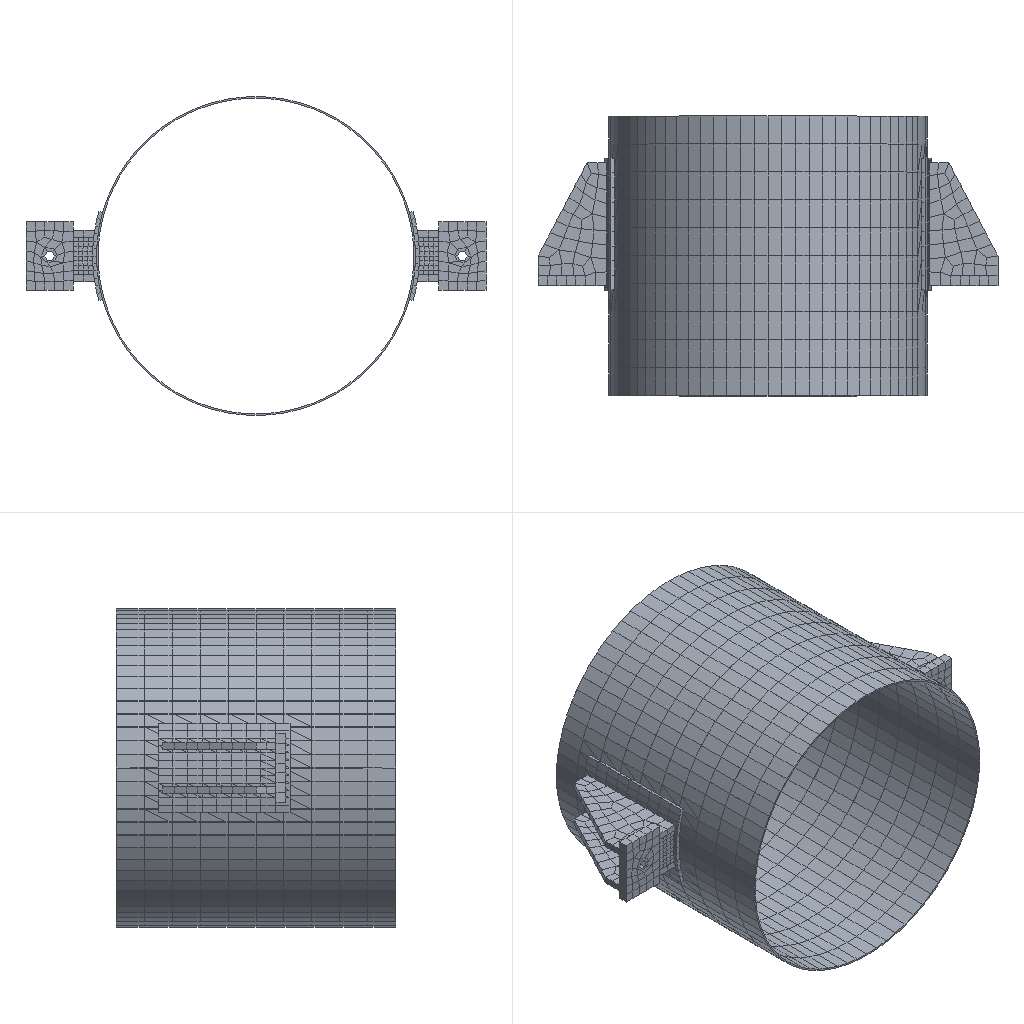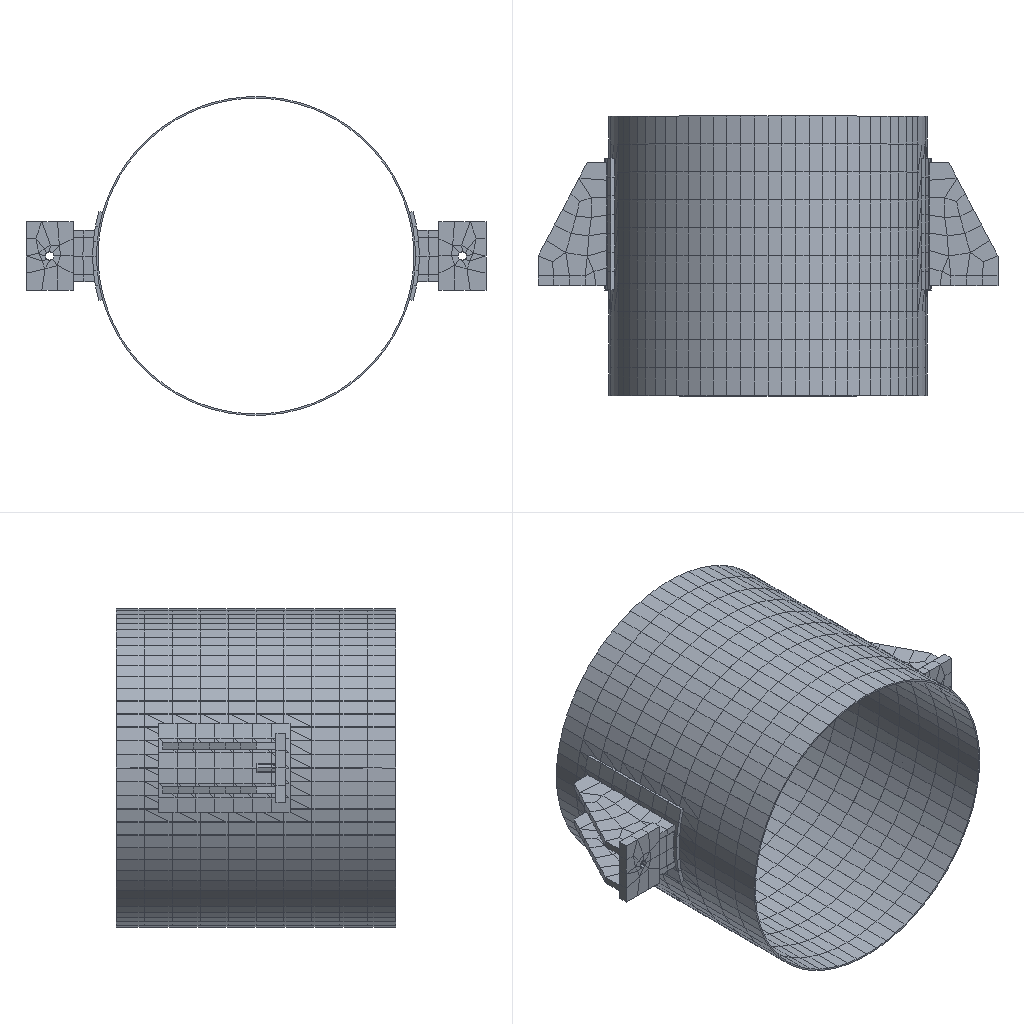Simulation study | ansys workbench
Set-up summary:
category,name,step,type,value,unit,region
solver,ansys_workbench
units,mm-N-s-tonne (MPa),,stated,"/units,MPA"
analysis,deck-1/LS1,,static
load_step,deck-1/LS1,deck-1/LS1,static,nsubst=1; time=1
analysis,deck-2/LS1,,static
load_step,deck-2/LS1,deck-2/LS1,static,nsubst=1; time=1
analysis,deck-3/LS1,,static
load_step,deck-3/LS1,deck-3/LS1,static,nsubst=1; time=1
mesh,deck-1.dat,,nodes,10142
mesh,deck-1.dat,,elements,2684
element_type,SOLID186,,,1302,,deck-1.dat
element_type,TARGE170,,,648,,deck-1.dat
element_type,CONTA174,,,648,,deck-1.dat
element_type,SURF154,,,86,,deck-1.dat
mesh,deck-2.dat,,nodes,10142
mesh,deck-2.dat,,elements,2684
element_type,SOLID186,,,1302,,deck-2.dat
element_type,TARGE170,,,648,,deck-2.dat
element_type,CONTA174,,,648,,deck-2.dat
element_type,SURF154,,,86,,deck-2.dat
mesh,deck-3.dat,,nodes,7696
mesh,deck-3.dat,,elements,1736
element_type,SOLID186,,,966,,deck-3.dat
element_type,TARGE170,,,364,,deck-3.dat
element_type,CONTA174,,,364,,deck-3.dat
element_type,SURF154,,,42,,deck-3.dat
material,Structural Steel,,E,200000,tonne s^-2 mm^-1
material,Structural Steel,,nu,0.3
material,Structural Steel,,density,7.85e-09,tonne mm^-3
material,Structural Steel,,conductivity,60.5,tonne mm s^-3 C^-1
material,Structural Steel,,specific_heat,4.34e+08,mm^2 s^-2 C^-1
material,Structural Steel,,cte,1.2e-05,C^-1
material,Structural Steel,,permeability,10000
material,Structural Steel,,resistivity,0.00017,ohm mm
material,Q355E,,E,200000,tonne s^-2 mm^-1
material,Q355E,,nu,0.3
material,Q355E,,density,7.85e-09,tonne mm^-3
material,Q355E,,conductivity,60.5,tonne mm s^-3 C^-1
material,Q355E,,specific_heat,4.34e+08,mm^2 s^-2 C^-1
material,Q355E,,cte,1.2e-05,C^-1
material,Q355E,,permeability,10000
material,Q355E,,resistivity,0.00017,ohm mm
load,Define Force Using Surface Effect Elements,deck-1/LS1,surface-effect pres face 2,0.9125,,SURF154 #48
load,Define Force Using Surface Effect Elements,deck-2/LS1,surface-effect pres face 2,3.65,,SURF154 #48
load,Define Force Using Surface Effect Elements,deck-3/LS1,surface-effect pres face 2,3.65,,SURF154 #54
bc,Fixed Supports,deck-1/model,fixed,[dofs=ALL],,_FIXEDSU
bc,Fixed Supports,deck-2/model,fixed,[dofs=ALL],,_FIXEDSU
bc,Fixed Supports,deck-3/model,fixed,[dofs=ALL],,_FIXEDSU
contact,Contact Region,,bonded (always),element=CONTA174
contact,Contact Region 2,,bonded (always),element=CONTA174
contact,Contact Region 3,,bonded (always),element=CONTA174
contact,Contact Region 4,,bonded (always),element=CONTA174
contact,Contact Region 5,,bonded (always),element=CONTA174
contact,Contact Region 6,,bonded (always),element=CONTA174
contact,Contact Region 7,,bonded (always),element=CONTA174
contact,Contact Region 8,,bonded (always),element=CONTA174
contact,Contact Region 9,,bonded (always),element=CONTA174
contact,Contact Region 10,,bonded (always),element=CONTA174
contact,Contact Region 11,,bonded (always),element=CONTA174
contact,Contact Region 12,,bonded (always),element=CONTA174
contact,Contact Region 13,,bonded (always),element=CONTA174
contact,Contact Region 14,,bonded (always),element=CONTA174
contact,Contact Region 15,,bonded (always),element=CONTA174
contact,Contact Region 16,,bonded (always),element=CONTA174
contact,Contact Region 17,,bonded (always),element=CONTA174
contact,Contact Region 18,,bonded (always),element=CONTA174
contact,Contact Region,,bonded (always),element=CONTA174
contact,Contact Region 2,,bonded (always),element=CONTA174
contact,Contact Region 3,,bonded (always),element=CONTA174
contact,Contact Region 4,,bonded (always),element=CONTA174
contact,Contact Region 5,,bonded (always),element=CONTA174
contact,Contact Region 6,,bonded (always),element=CONTA174
contact,Contact Region 7,,bonded (always),element=CONTA174
contact,Contact Region 8,,bonded (always),element=CONTA174
contact,Contact Region 9,,bonded (always),element=CONTA174
contact,Contact Region 10,,bonded (always),element=CONTA174
contact,Contact Region 11,,bonded (always),element=CONTA174
contact,Contact Region 12,,bonded (always),element=CONTA174
contact,Contact Region 13,,bonded (always),element=CONTA174
contact,Contact Region 14,,bonded (always),element=CONTA174
contact,Contact Region 15,,bonded (always),element=CONTA174
contact,Contact Region 16,,bonded (always),element=CONTA174
contact,Contact Region 17,,bonded (always),element=CONTA174
contact,Contact Region 18,,bonded (always),element=CONTA174
contact,Contact Region,,bonded (always),element=CONTA174
contact,Contact Region 2,,bonded (always),element=CONTA174
contact,Contact Region 3,,bonded (always),element=CONTA174
contact,Contact Region 4,,bonded (always),element=CONTA174
contact,Contact Region 5,,bonded (always),element=CONTA174
contact,Contact Region 6,,bonded (always),element=CONTA174
contact,Contact Region 7,,bonded (always),element=CONTA174
contact,Contact Region 8,,bonded (always),element=CONTA174
contact,Contact Region 9,,bonded (always),element=CONTA174
contact,Contact Region 10,,bonded (always),element=CONTA174
contact,Contact Region 11,,bonded (always),element=CONTA174
contact,Contact Region 12,,bonded (always),element=CONTA174
contact,Contact Region 13,,bonded (always),element=CONTA174
contact,Contact Region 14,,bonded (always),element=CONTA174
contact,Contact Region 15,,bonded (always),element=CONTA174
contact,Contact Region 16,,bonded (always),element=CONTA174
contact,Contact Region 17,,bonded (always),element=CONTA174
contact,Contact Region 18,,bonded (always),element=CONTA174
contact,Contact Region 19,,bonded (always),element=CONTA174
contact,Contact Region 20,,bonded (always),element=CONTA174
named_set,_FIXEDSU,,node,60
named_set,_FIXEDSU,,node,60
named_set,______,,node,208
named_set,_FIXEDSU,,node,208
Results summary:
result,analyses[0].index,,,1
result,analyses[0].system,,,SYS
result,analyses[0].deck,,,deck-1.dat
result,analyses[0].solve_status,,,completed
result,analyses[0].analysis_type,,,static
result,analyses[0].physics,,,mechanical
result,analyses[0].unit_system,,,"NMM: mm, ton, N, s, mV, mA, degC"
result,analyses[0].n_sets,,,1
result,analyses[0].load_steps[0].set,set=1,,1
result,analyses[0].load_steps[0].time_or_freq,set=1,,1
result,analyses[0].load_steps[0].max_displacement_magnitude,set=1,,0.03549
result,analyses[0].load_steps[0].max_von_mises_nodal,set=1,,41.627
result,analyses[0].load_steps[0].reaction_force_sum_xyz[1],set=1,,-2.22756e-06
result,analyses[0].load_steps[0].reaction_force_sum_xyz[2],set=1,,-150000
result,analyses[0].load_steps[0].reaction_force_sum_xyz[3],set=1,,7.2564e-08
result,analyses[1].index,,,2
result,analyses[1].system,,,SYS-1
result,analyses[1].deck,,,deck-2.dat
result,analyses[1].solve_status,,,completed
result,analyses[1].analysis_type,,,static
result,analyses[1].physics,,,mechanical
result,analyses[1].unit_system,,,"NMM: mm, ton, N, s, mV, mA, degC"
result,analyses[1].n_sets,,,1
result,analyses[1].load_steps[0].set,set=1,,1
result,analyses[1].load_steps[0].time_or_freq,set=1,,1
result,analyses[1].load_steps[0].max_displacement_magnitude,set=1,,0.142
result,analyses[1].load_steps[0].max_von_mises_nodal,set=1,,166.509
result,analyses[1].load_steps[0].reaction_force_sum_xyz[1],set=1,,-8.91031e-06
result,analyses[1].load_steps[0].reaction_force_sum_xyz[2],set=1,,-600000
result,analyses[1].load_steps[0].reaction_force_sum_xyz[3],set=1,,2.8978e-07
result,analyses[2].index,,,3
result,analyses[2].system,,,SYS-2
result,analyses[2].deck,,,deck-3.dat
result,analyses[2].solve_status,,,completed
result,analyses[2].analysis_type,,,static
result,analyses[2].physics,,,mechanical
result,analyses[2].unit_system,,,"NMM: mm, ton, N, s, mV, mA, degC"
result,analyses[2].n_sets,,,1
result,analyses[2].load_steps[0].set,set=1,,1
result,analyses[2].load_steps[0].time_or_freq,set=1,,1
result,analyses[2].load_steps[0].max_displacement_magnitude,set=1,,0.137
result,analyses[2].load_steps[0].max_von_mises_nodal,set=1,,136.407
result,analyses[2].load_steps[0].reaction_force_sum_xyz[1],set=1,,-7.19499e-06
result,analyses[2].load_steps[0].reaction_force_sum_xyz[2],set=1,,-600000
result,analyses[2].load_steps[0].reaction_force_sum_xyz[3],set=1,,5.74828e-08
result,geometry_export[0][0],,,.step
result,geometry_export[0][1],,,ok
result,geometry_export[0][2],,,11